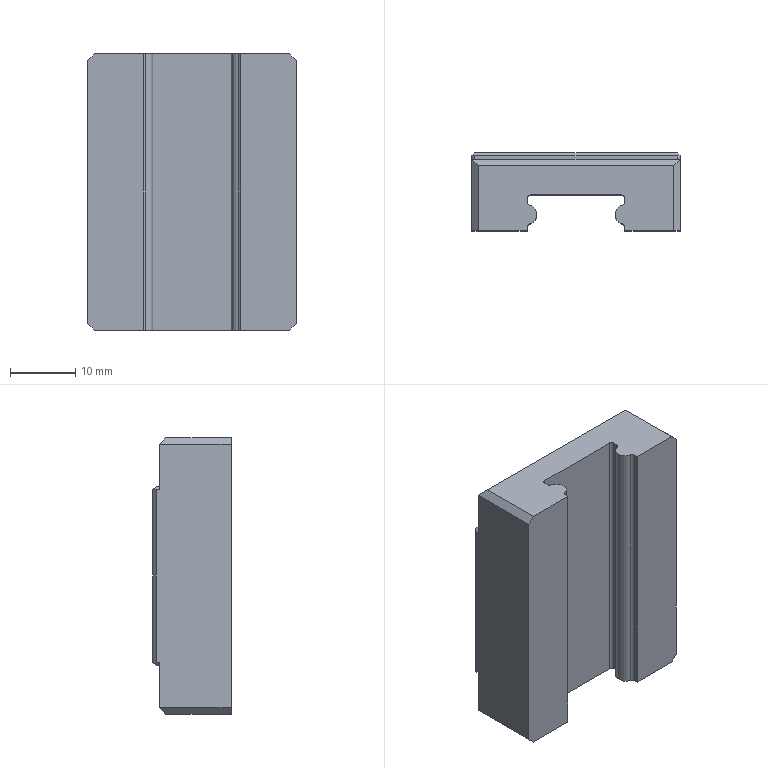Part | STEP file | PN_0016 | 1 solid | 58 faces | box 32 x 12 x 42.4 mm | volume 12345 mm3 | plane 34 | cylinder 16 | cone 8 | commonest cylinder face diameters 2.5 x8 1 x6 3 x2